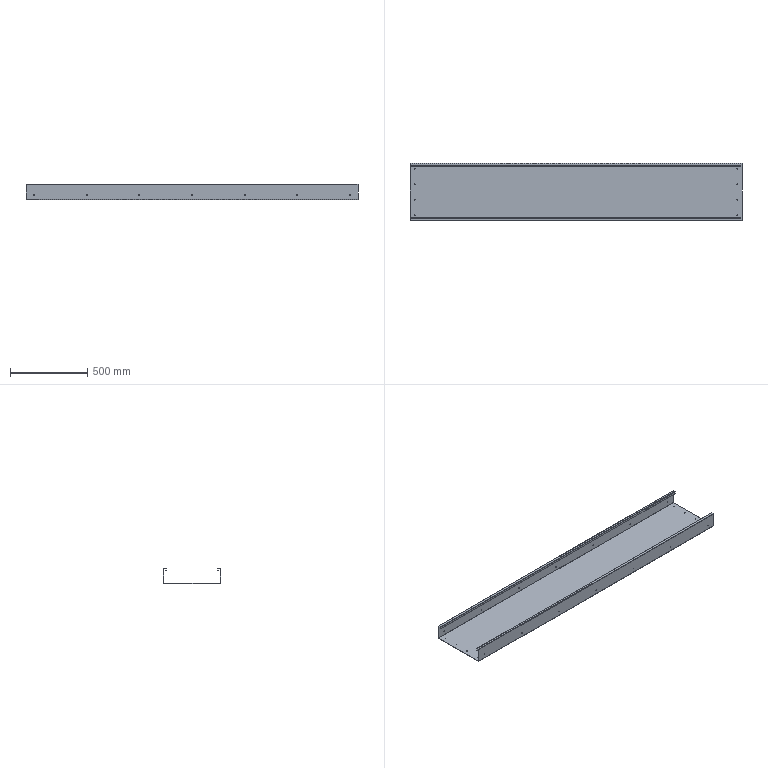Part | STEP file | TS-S13 | 1 solid | 98 faces | box 2145 x 370 x 97 mm | volume 2636955 mm3 | cylinder 56 | plane 42 | commonest cylinder face diameters 5.4 x44 0.4 x6 4.4 x6